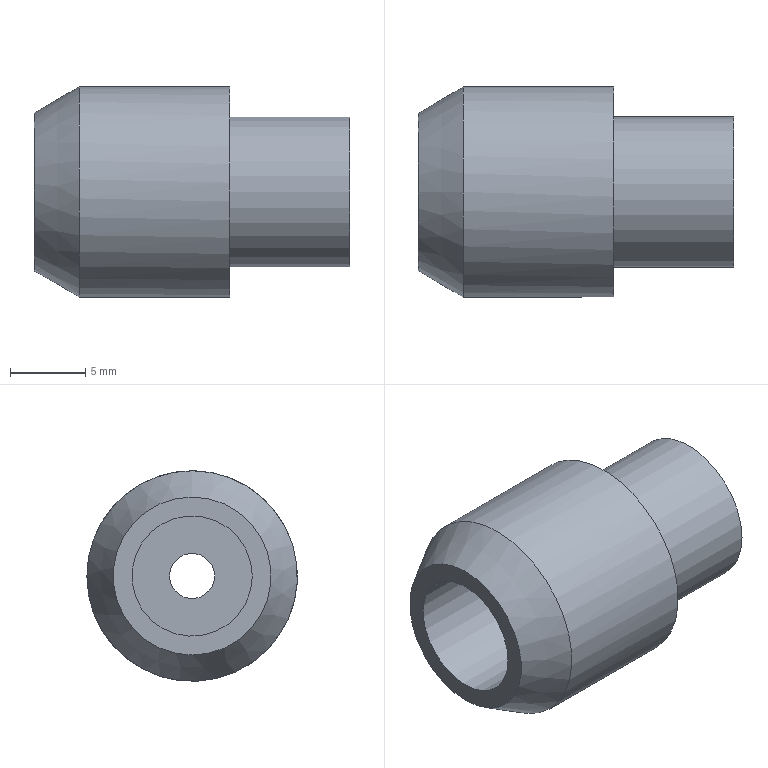Part | STEP file | 1-23.3 | 1 solid | 9 faces | box 21 x 14 x 14 mm | volume 1943 mm3 | cylinder 4 | plane 4 | cone 1 | commonest cylinder face diameters 3 x1 8 x1 10 x1 14 x1
STEP:
#1=CARTESIAN_POINT('',(0.,0.,0.));
#2=DIRECTION('',(0.,0.,1.));
#3=DIRECTION('',(1.,0.,0.));
#4=AXIS2_PLACEMENT_3D('',#1,#2,#3);
#5=CARTESIAN_POINT('',(0.,7.,0.));
#6=VERTEX_POINT('',#5);
#7=CARTESIAN_POINT('',(-10.,7.,0.));
#8=VERTEX_POINT('',#7);
#9=CARTESIAN_POINT('',(0.,7.,0.));
#10=DIRECTION('',(-1.,0.,0.));
#11=VECTOR('',#10,1.);
#12=LINE('',#9,#11);
#13=CARTESIAN_POINT('',(0.,0.,0.));
#14=DIRECTION('',(-1.,0.,0.));
#15=DIRECTION('',(0.,1.,0.));
#16=AXIS2_PLACEMENT_3D('',#13,#14,#15);
#17=CYLINDRICAL_SURFACE('',#16,7.);
#18=CARTESIAN_POINT('',(6.283,0.));
#19=DIRECTION('',(0.,1.));
#20=VECTOR('',#19,1.);
#21=LINE('',#18,#20);
#22=(GEOMETRIC_REPRESENTATION_CONTEXT(2)PARAMETRIC_REPRESENTATION_CONTEXT()REPRESENTATION_CONTEXT('',''));
#23=DEFINITIONAL_REPRESENTATION('',(#21),#22);
#24=PCURVE('',#17,#23);
#25=CARTESIAN_POINT('',(0.,0.));
#26=DIRECTION('',(0.,1.));
#27=VECTOR('',#26,1.);
#28=LINE('',#25,#27);
#29=(GEOMETRIC_REPRESENTATION_CONTEXT(2)PARAMETRIC_REPRESENTATION_CONTEXT()REPRESENTATION_CONTEXT('',''));
#30=DEFINITIONAL_REPRESENTATION('',(#28),#29);
#31=PCURVE('',#17,#30);
#32=SEAM_CURVE('',#12,(#24,#31),.PCURVE_S1.);
#33=EDGE_CURVE('',#6,#8,#32,.T.);
#34=ORIENTED_EDGE('',*,*,#33,.T.);
#35=CARTESIAN_POINT('',(-10.,0.,7.));
#36=VERTEX_POINT('',#35);
#37=CARTESIAN_POINT('',(-10.,0.,0.));
#38=DIRECTION('',(1.,0.,0.));
#39=DIRECTION('',(0.,1.,0.));
#40=AXIS2_PLACEMENT_3D('',#37,#38,#39);
#41=CIRCLE('',#40,7.);
#42=CARTESIAN_POINT('',(6.283,10.));
#43=DIRECTION('',(-1.,0.));
#44=VECTOR('',#43,1.);
#45=LINE('',#42,#44);
#46=(GEOMETRIC_REPRESENTATION_CONTEXT(2)PARAMETRIC_REPRESENTATION_CONTEXT()REPRESENTATION_CONTEXT('',''));
#47=DEFINITIONAL_REPRESENTATION('',(#45),#46);
#48=PCURVE('',#17,#47);
#49=CARTESIAN_POINT('',(-13.,0.,0.));
#50=DIRECTION('',(1.,0.,0.));
#51=DIRECTION('',(0.,0.,1.));
#52=AXIS2_PLACEMENT_3D('',#49,#50,#51);
#53=CONICAL_SURFACE('',#52,5.25,0.5281);
#54=CARTESIAN_POINT('',(4.712,3.));
#55=DIRECTION('',(1.,0.));
#56=VECTOR('',#55,1.);
#57=LINE('',#54,#56);
#58=(GEOMETRIC_REPRESENTATION_CONTEXT(2)PARAMETRIC_REPRESENTATION_CONTEXT()REPRESENTATION_CONTEXT('',''));
#59=DEFINITIONAL_REPRESENTATION('',(#57),#58);
#60=PCURVE('',#53,#59);
#61=SURFACE_CURVE('',#41,(#48,#60),.PCURVE_S1.);
#62=EDGE_CURVE('',#8,#36,#61,.T.);
#63=ORIENTED_EDGE('',*,*,#62,.T.);
#64=CARTESIAN_POINT('',(-10.,0.,0.));
#65=DIRECTION('',(1.,0.,0.));
#66=DIRECTION('',(0.,0.,1.));
#67=AXIS2_PLACEMENT_3D('',#64,#65,#66);
#68=CIRCLE('',#67,7.);
#69=CARTESIAN_POINT('',(4.712,10.));
#70=DIRECTION('',(-1.,0.));
#71=VECTOR('',#70,1.);
#72=LINE('',#69,#71);
#73=(GEOMETRIC_REPRESENTATION_CONTEXT(2)PARAMETRIC_REPRESENTATION_CONTEXT()REPRESENTATION_CONTEXT('',''));
#74=DEFINITIONAL_REPRESENTATION('',(#72),#73);
#75=PCURVE('',#17,#74);
#76=CARTESIAN_POINT('',(0.,3.));
#77=DIRECTION('',(1.,0.));
#78=VECTOR('',#77,1.);
#79=LINE('',#76,#78);
#80=(GEOMETRIC_REPRESENTATION_CONTEXT(2)PARAMETRIC_REPRESENTATION_CONTEXT()REPRESENTATION_CONTEXT('',''));
#81=DEFINITIONAL_REPRESENTATION('',(#79),#80);
#82=PCURVE('',#53,#81);
#83=SURFACE_CURVE('',#68,(#75,#82),.PCURVE_S1.);
#84=EDGE_CURVE('',#36,#8,#83,.T.);
#85=ORIENTED_EDGE('',*,*,#84,.T.);
#86=ORIENTED_EDGE('',*,*,#33,.F.);
#87=CARTESIAN_POINT('',(0.,0.,0.));
#88=DIRECTION('',(1.,0.,0.));
#89=DIRECTION('',(0.,1.,0.));
#90=AXIS2_PLACEMENT_3D('',#87,#88,#89);
#91=CIRCLE('',#90,7.);
#92=CARTESIAN_POINT('',(6.283,0.));
#93=DIRECTION('',(-1.,0.));
#94=VECTOR('',#93,1.);
#95=LINE('',#92,#94);
#96=(GEOMETRIC_REPRESENTATION_CONTEXT(2)PARAMETRIC_REPRESENTATION_CONTEXT()REPRESENTATION_CONTEXT('',''));
#97=DEFINITIONAL_REPRESENTATION('',(#95),#96);
#98=PCURVE('',#17,#97);
#99=CARTESIAN_POINT('',(0.,-1.876,0.));
#100=DIRECTION('',(1.,0.,0.));
#101=DIRECTION('',(0.,0.,-1.));
#102=AXIS2_PLACEMENT_3D('',#99,#100,#101);
#103=PLANE('',#102);
#104=CARTESIAN_POINT('',(0.,1.876));
#105=DIRECTION('',(0.,1.));
#106=AXIS2_PLACEMENT_2D('',#104,#105);
#107=CIRCLE('',#106,7.);
#108=(GEOMETRIC_REPRESENTATION_CONTEXT(2)PARAMETRIC_REPRESENTATION_CONTEXT()REPRESENTATION_CONTEXT('',''));
#109=DEFINITIONAL_REPRESENTATION('',(#107),#108);
#110=PCURVE('',#103,#109);
#111=SURFACE_CURVE('',#91,(#98,#110),.PCURVE_S1.);
#112=EDGE_CURVE('',#6,#6,#111,.T.);
#113=ORIENTED_EDGE('',*,*,#112,.F.);
#114=EDGE_LOOP('',(#34,#63,#85,#86,#113));
#115=FACE_BOUND('',#114,.T.);
#116=ADVANCED_FACE('',(#115),#17,.T.);
#117=ORIENTED_EDGE('',*,*,#112,.T.);
#118=EDGE_LOOP('',(#117));
#119=FACE_BOUND('',#118,.T.);
#120=CARTESIAN_POINT('',(0.,5.,0.));
#121=VERTEX_POINT('',#120);
#122=CARTESIAN_POINT('',(0.,0.,0.));
#123=DIRECTION('',(1.,0.,0.));
#124=DIRECTION('',(0.,1.,0.));
#125=AXIS2_PLACEMENT_3D('',#122,#123,#124);
#126=CIRCLE('',#125,5.);
#127=CARTESIAN_POINT('',(0.,1.876));
#128=DIRECTION('',(0.,1.));
#129=AXIS2_PLACEMENT_2D('',#127,#128);
#130=CIRCLE('',#129,5.);
#131=(GEOMETRIC_REPRESENTATION_CONTEXT(2)PARAMETRIC_REPRESENTATION_CONTEXT()REPRESENTATION_CONTEXT('',''));
#132=DEFINITIONAL_REPRESENTATION('',(#130),#131);
#133=PCURVE('',#103,#132);
#134=CARTESIAN_POINT('',(0.,0.,0.));
#135=DIRECTION('',(1.,0.,0.));
#136=DIRECTION('',(0.,1.,0.));
#137=AXIS2_PLACEMENT_3D('',#134,#135,#136);
#138=CYLINDRICAL_SURFACE('',#137,5.);
#139=CARTESIAN_POINT('',(0.,0.));
#140=DIRECTION('',(1.,0.));
#141=VECTOR('',#140,1.);
#142=LINE('',#139,#141);
#143=(GEOMETRIC_REPRESENTATION_CONTEXT(2)PARAMETRIC_REPRESENTATION_CONTEXT()REPRESENTATION_CONTEXT('',''));
#144=DEFINITIONAL_REPRESENTATION('',(#142),#143);
#145=PCURVE('',#138,#144);
#146=SURFACE_CURVE('',#126,(#133,#145),.PCURVE_S1.);
#147=EDGE_CURVE('',#121,#121,#146,.T.);
#148=ORIENTED_EDGE('',*,*,#147,.F.);
#149=EDGE_LOOP('',(#148));
#150=FACE_BOUND('',#149,.T.);
#151=ADVANCED_FACE('',(#119,#150),#103,.T.);
#152=ORIENTED_EDGE('',*,*,#147,.T.);
#153=CARTESIAN_POINT('',(8.,5.,0.));
#154=VERTEX_POINT('',#153);
#155=CARTESIAN_POINT('',(0.,5.,0.));
#156=DIRECTION('',(1.,0.,0.));
#157=VECTOR('',#156,1.);
#158=LINE('',#155,#157);
#159=CARTESIAN_POINT('',(6.283,0.));
#160=DIRECTION('',(0.,1.));
#161=VECTOR('',#160,1.);
#162=LINE('',#159,#161);
#163=(GEOMETRIC_REPRESENTATION_CONTEXT(2)PARAMETRIC_REPRESENTATION_CONTEXT()REPRESENTATION_CONTEXT('',''));
#164=DEFINITIONAL_REPRESENTATION('',(#162),#163);
#165=PCURVE('',#138,#164);
#166=CARTESIAN_POINT('',(0.,0.));
#167=DIRECTION('',(0.,1.));
#168=VECTOR('',#167,1.);
#169=LINE('',#166,#168);
#170=(GEOMETRIC_REPRESENTATION_CONTEXT(2)PARAMETRIC_REPRESENTATION_CONTEXT()REPRESENTATION_CONTEXT('',''));
#171=DEFINITIONAL_REPRESENTATION('',(#169),#170);
#172=PCURVE('',#138,#171);
#173=SEAM_CURVE('',#158,(#165,#172),.PCURVE_S1.);
#174=EDGE_CURVE('',#121,#154,#173,.T.);
#175=ORIENTED_EDGE('',*,*,#174,.T.);
#176=CARTESIAN_POINT('',(8.,0.,0.));
#177=DIRECTION('',(1.,0.,0.));
#178=DIRECTION('',(0.,1.,0.));
#179=AXIS2_PLACEMENT_3D('',#176,#177,#178);
#180=CIRCLE('',#179,5.);
#181=CARTESIAN_POINT('',(0.,8.));
#182=DIRECTION('',(1.,0.));
#183=VECTOR('',#182,1.);
#184=LINE('',#181,#183);
#185=(GEOMETRIC_REPRESENTATION_CONTEXT(2)PARAMETRIC_REPRESENTATION_CONTEXT()REPRESENTATION_CONTEXT('',''));
#186=DEFINITIONAL_REPRESENTATION('',(#184),#185);
#187=PCURVE('',#138,#186);
#188=CARTESIAN_POINT('',(8.,-1.34,0.));
#189=DIRECTION('',(1.,0.,0.));
#190=DIRECTION('',(0.,0.,-1.));
#191=AXIS2_PLACEMENT_3D('',#188,#189,#190);
#192=PLANE('',#191);
#193=CARTESIAN_POINT('',(0.,1.34));
#194=DIRECTION('',(0.,1.));
#195=AXIS2_PLACEMENT_2D('',#193,#194);
#196=CIRCLE('',#195,5.);
#197=(GEOMETRIC_REPRESENTATION_CONTEXT(2)PARAMETRIC_REPRESENTATION_CONTEXT()REPRESENTATION_CONTEXT('',''));
#198=DEFINITIONAL_REPRESENTATION('',(#196),#197);
#199=PCURVE('',#192,#198);
#200=SURFACE_CURVE('',#180,(#187,#199),.PCURVE_S1.);
#201=EDGE_CURVE('',#154,#154,#200,.T.);
#202=ORIENTED_EDGE('',*,*,#201,.F.);
#203=ORIENTED_EDGE('',*,*,#174,.F.);
#204=EDGE_LOOP('',(#152,#175,#202,#203));
#205=FACE_BOUND('',#204,.T.);
#206=ADVANCED_FACE('',(#205),#138,.T.);
#207=ORIENTED_EDGE('',*,*,#62,.F.);
#208=ORIENTED_EDGE('',*,*,#84,.F.);
#209=CARTESIAN_POINT('',(-13.,0.,5.25));
#210=VERTEX_POINT('',#209);
#211=CARTESIAN_POINT('',(-10.,0.,7.));
#212=DIRECTION('',(-0.8638,0.,-0.5039));
#213=VECTOR('',#212,1.);
#214=LINE('',#211,#213);
#215=CARTESIAN_POINT('',(0.,3.));
#216=DIRECTION('',(0.,-1.));
#217=VECTOR('',#216,1.);
#218=LINE('',#215,#217);
#219=(GEOMETRIC_REPRESENTATION_CONTEXT(2)PARAMETRIC_REPRESENTATION_CONTEXT()REPRESENTATION_CONTEXT('',''));
#220=DEFINITIONAL_REPRESENTATION('',(#218),#219);
#221=PCURVE('',#53,#220);
#222=CARTESIAN_POINT('',(6.283,3.));
#223=DIRECTION('',(0.,-1.));
#224=VECTOR('',#223,1.);
#225=LINE('',#222,#224);
#226=(GEOMETRIC_REPRESENTATION_CONTEXT(2)PARAMETRIC_REPRESENTATION_CONTEXT()REPRESENTATION_CONTEXT('',''));
#227=DEFINITIONAL_REPRESENTATION('',(#225),#226);
#228=PCURVE('',#53,#227);
#229=SEAM_CURVE('',#214,(#221,#228),.PCURVE_S1.);
#230=EDGE_CURVE('',#36,#210,#229,.T.);
#231=ORIENTED_EDGE('',*,*,#230,.T.);
#232=CARTESIAN_POINT('',(-13.,0.,0.));
#233=DIRECTION('',(-1.,0.,0.));
#234=DIRECTION('',(0.,0.,1.));
#235=AXIS2_PLACEMENT_3D('',#232,#233,#234);
#236=CIRCLE('',#235,5.25);
#237=CARTESIAN_POINT('',(6.283,0.));
#238=DIRECTION('',(-1.,0.));
#239=VECTOR('',#238,1.);
#240=LINE('',#237,#239);
#241=(GEOMETRIC_REPRESENTATION_CONTEXT(2)PARAMETRIC_REPRESENTATION_CONTEXT()REPRESENTATION_CONTEXT('',''));
#242=DEFINITIONAL_REPRESENTATION('',(#240),#241);
#243=PCURVE('',#53,#242);
#244=CARTESIAN_POINT('',(-13.,0.,0.));
#245=DIRECTION('',(1.,0.,0.));
#246=DIRECTION('',(0.,0.,1.));
#247=AXIS2_PLACEMENT_3D('',#244,#245,#246);
#248=PLANE('',#247);
#249=CARTESIAN_POINT('',(5.25,0.));
#250=CARTESIAN_POINT('',(5.25,-9.093));
#251=CARTESIAN_POINT('',(-2.625,-4.547));
#252=CARTESIAN_POINT('',(-10.5,0.));
#253=CARTESIAN_POINT('',(-2.625,4.547));
#254=CARTESIAN_POINT('',(5.25,9.093));
#255=CARTESIAN_POINT('',(5.25,0.));
#256=(BOUNDED_CURVE()B_SPLINE_CURVE(2,(#249,#250,#251,#252,#253,#254,#255),.UNSPECIFIED.,.T.,.F.)B_SPLINE_CURVE_WITH_KNOTS((1,2,2,2,2,1),(-2.094,0.,2.094,4.189,6.283,8.378),.UNSPECIFIED.)CURVE()GEOMETRIC_REPRESENTATION_ITEM()RATIONAL_B_SPLINE_CURVE((1.,0.5,1.,0.5,1.,0.5,1.))REPRESENTATION_ITEM(''));
#257=(GEOMETRIC_REPRESENTATION_CONTEXT(2)PARAMETRIC_REPRESENTATION_CONTEXT()REPRESENTATION_CONTEXT('',''));
#258=DEFINITIONAL_REPRESENTATION('',(#256),#257);
#259=PCURVE('',#248,#258);
#260=SURFACE_CURVE('',#236,(#243,#259),.PCURVE_S1.);
#261=EDGE_CURVE('',#210,#210,#260,.T.);
#262=ORIENTED_EDGE('',*,*,#261,.F.);
#263=ORIENTED_EDGE('',*,*,#230,.F.);
#264=EDGE_LOOP('',(#207,#208,#231,#262,#263));
#265=FACE_BOUND('',#264,.T.);
#266=ADVANCED_FACE('',(#265),#53,.T.);
#267=ORIENTED_EDGE('',*,*,#261,.F.);
#268=EDGE_LOOP('',(#267));
#269=FACE_BOUND('',#268,.F.);
#270=CARTESIAN_POINT('',(-13.,-4.,0.));
#271=VERTEX_POINT('',#270);
#272=CARTESIAN_POINT('',(-13.,0.,0.));
#273=DIRECTION('',(-1.,0.,0.));
#274=DIRECTION('',(0.,-1.,0.));
#275=AXIS2_PLACEMENT_3D('',#272,#273,#274);
#276=CIRCLE('',#275,4.);
#277=CARTESIAN_POINT('',(0.,4.));
#278=CARTESIAN_POINT('',(6.928,4.));
#279=CARTESIAN_POINT('',(3.464,-2.));
#280=CARTESIAN_POINT('',(0.,-8.));
#281=CARTESIAN_POINT('',(-3.464,-2.));
#282=CARTESIAN_POINT('',(-6.928,4.));
#283=CARTESIAN_POINT('',(0.,4.));
#284=(BOUNDED_CURVE()B_SPLINE_CURVE(2,(#277,#278,#279,#280,#281,#282,#283),.UNSPECIFIED.,.T.,.F.)B_SPLINE_CURVE_WITH_KNOTS((1,2,2,2,2,1),(-2.094,0.,2.094,4.189,6.283,8.378),.UNSPECIFIED.)CURVE()GEOMETRIC_REPRESENTATION_ITEM()RATIONAL_B_SPLINE_CURVE((1.,0.5,1.,0.5,1.,0.5,1.))REPRESENTATION_ITEM(''));
#285=(GEOMETRIC_REPRESENTATION_CONTEXT(2)PARAMETRIC_REPRESENTATION_CONTEXT()REPRESENTATION_CONTEXT('',''));
#286=DEFINITIONAL_REPRESENTATION('',(#284),#285);
#287=PCURVE('',#248,#286);
#288=CARTESIAN_POINT('',(-13.,0.,0.));
#289=DIRECTION('',(1.,0.,0.));
#290=DIRECTION('',(0.,-1.,0.));
#291=AXIS2_PLACEMENT_3D('',#288,#289,#290);
#292=CYLINDRICAL_SURFACE('',#291,4.);
#293=CARTESIAN_POINT('',(6.283,0.));
#294=DIRECTION('',(-1.,0.));
#295=VECTOR('',#294,1.);
#296=LINE('',#293,#295);
#297=(GEOMETRIC_REPRESENTATION_CONTEXT(2)PARAMETRIC_REPRESENTATION_CONTEXT()REPRESENTATION_CONTEXT('',''));
#298=DEFINITIONAL_REPRESENTATION('',(#296),#297);
#299=PCURVE('',#292,#298);
#300=SURFACE_CURVE('',#276,(#287,#299),.PCURVE_S1.);
#301=EDGE_CURVE('',#271,#271,#300,.T.);
#302=ORIENTED_EDGE('',*,*,#301,.T.);
#303=EDGE_LOOP('',(#302));
#304=FACE_BOUND('',#303,.F.);
#305=ADVANCED_FACE('',(#269,#304),#248,.F.);
#306=CARTESIAN_POINT('',(-3.,-4.,0.));
#307=VERTEX_POINT('',#306);
#308=CARTESIAN_POINT('',(-13.,-4.,0.));
#309=DIRECTION('',(1.,0.,0.));
#310=VECTOR('',#309,1.);
#311=LINE('',#308,#310);
#312=CARTESIAN_POINT('',(6.283,0.));
#313=DIRECTION('',(0.,1.));
#314=VECTOR('',#313,1.);
#315=LINE('',#312,#314);
#316=(GEOMETRIC_REPRESENTATION_CONTEXT(2)PARAMETRIC_REPRESENTATION_CONTEXT()REPRESENTATION_CONTEXT('',''));
#317=DEFINITIONAL_REPRESENTATION('',(#315),#316);
#318=PCURVE('',#292,#317);
#319=CARTESIAN_POINT('',(0.,0.));
#320=DIRECTION('',(0.,1.));
#321=VECTOR('',#320,1.);
#322=LINE('',#319,#321);
#323=(GEOMETRIC_REPRESENTATION_CONTEXT(2)PARAMETRIC_REPRESENTATION_CONTEXT()REPRESENTATION_CONTEXT('',''));
#324=DEFINITIONAL_REPRESENTATION('',(#322),#323);
#325=PCURVE('',#292,#324);
#326=SEAM_CURVE('',#311,(#318,#325),.PCURVE_S1.);
#327=EDGE_CURVE('',#271,#307,#326,.T.);
#328=ORIENTED_EDGE('',*,*,#327,.T.);
#329=CARTESIAN_POINT('',(-3.,0.,0.));
#330=DIRECTION('',(-1.,0.,0.));
#331=DIRECTION('',(0.,-1.,0.));
#332=AXIS2_PLACEMENT_3D('',#329,#330,#331);
#333=CIRCLE('',#332,4.);
#334=CARTESIAN_POINT('',(6.283,10.));
#335=DIRECTION('',(-1.,0.));
#336=VECTOR('',#335,1.);
#337=LINE('',#334,#336);
#338=(GEOMETRIC_REPRESENTATION_CONTEXT(2)PARAMETRIC_REPRESENTATION_CONTEXT()REPRESENTATION_CONTEXT('',''));
#339=DEFINITIONAL_REPRESENTATION('',(#337),#338);
#340=PCURVE('',#292,#339);
#341=CARTESIAN_POINT('',(-3.,1.072,0.));
#342=DIRECTION('',(-1.,0.,0.));
#343=DIRECTION('',(0.,-1.,0.));
#344=AXIS2_PLACEMENT_3D('',#341,#342,#343);
#345=PLANE('',#344);
#346=CARTESIAN_POINT('',(1.072,0.));
#347=DIRECTION('',(1.,0.));
#348=AXIS2_PLACEMENT_2D('',#346,#347);
#349=CIRCLE('',#348,4.);
#350=(GEOMETRIC_REPRESENTATION_CONTEXT(2)PARAMETRIC_REPRESENTATION_CONTEXT()REPRESENTATION_CONTEXT('',''));
#351=DEFINITIONAL_REPRESENTATION('',(#349),#350);
#352=PCURVE('',#345,#351);
#353=SURFACE_CURVE('',#333,(#340,#352),.PCURVE_S1.);
#354=EDGE_CURVE('',#307,#307,#353,.T.);
#355=ORIENTED_EDGE('',*,*,#354,.T.);
#356=ORIENTED_EDGE('',*,*,#327,.F.);
#357=ORIENTED_EDGE('',*,*,#301,.F.);
#358=EDGE_LOOP('',(#328,#355,#356,#357));
#359=FACE_BOUND('',#358,.F.);
#360=ADVANCED_FACE('',(#359),#292,.F.);
#361=ORIENTED_EDGE('',*,*,#201,.T.);
#362=EDGE_LOOP('',(#361));
#363=FACE_BOUND('',#362,.T.);
#364=CARTESIAN_POINT('',(8.,1.5,0.));
#365=VERTEX_POINT('',#364);
#366=CARTESIAN_POINT('',(8.,0.,0.));
#367=DIRECTION('',(1.,0.,0.));
#368=DIRECTION('',(0.,1.,0.));
#369=AXIS2_PLACEMENT_3D('',#366,#367,#368);
#370=CIRCLE('',#369,1.5);
#371=CARTESIAN_POINT('',(0.,1.34));
#372=DIRECTION('',(0.,1.));
#373=AXIS2_PLACEMENT_2D('',#371,#372);
#374=CIRCLE('',#373,1.5);
#375=(GEOMETRIC_REPRESENTATION_CONTEXT(2)PARAMETRIC_REPRESENTATION_CONTEXT()REPRESENTATION_CONTEXT('',''));
#376=DEFINITIONAL_REPRESENTATION('',(#374),#375);
#377=PCURVE('',#192,#376);
#378=CARTESIAN_POINT('',(8.,0.,0.));
#379=DIRECTION('',(-1.,0.,0.));
#380=DIRECTION('',(0.,1.,0.));
#381=AXIS2_PLACEMENT_3D('',#378,#379,#380);
#382=CYLINDRICAL_SURFACE('',#381,1.5);
#383=CARTESIAN_POINT('',(6.283,0.));
#384=DIRECTION('',(-1.,0.));
#385=VECTOR('',#384,1.);
#386=LINE('',#383,#385);
#387=(GEOMETRIC_REPRESENTATION_CONTEXT(2)PARAMETRIC_REPRESENTATION_CONTEXT()REPRESENTATION_CONTEXT('',''));
#388=DEFINITIONAL_REPRESENTATION('',(#386),#387);
#389=PCURVE('',#382,#388);
#390=SURFACE_CURVE('',#370,(#377,#389),.PCURVE_S1.);
#391=EDGE_CURVE('',#365,#365,#390,.T.);
#392=ORIENTED_EDGE('',*,*,#391,.F.);
#393=EDGE_LOOP('',(#392));
#394=FACE_BOUND('',#393,.T.);
#395=ADVANCED_FACE('',(#363,#394),#192,.T.);
#396=ORIENTED_EDGE('',*,*,#354,.T.);
#397=EDGE_LOOP('',(#396));
#398=FACE_BOUND('',#397,.T.);
#399=CARTESIAN_POINT('',(-3.,1.5,0.));
#400=VERTEX_POINT('',#399);
#401=CARTESIAN_POINT('',(-3.,0.,0.));
#402=DIRECTION('',(-1.,0.,0.));
#403=DIRECTION('',(0.,1.,0.));
#404=AXIS2_PLACEMENT_3D('',#401,#402,#403);
#405=CIRCLE('',#404,1.5);
#406=CARTESIAN_POINT('',(1.072,0.));
#407=DIRECTION('',(-1.,0.));
#408=AXIS2_PLACEMENT_2D('',#406,#407);
#409=CIRCLE('',#408,1.5);
#410=(GEOMETRIC_REPRESENTATION_CONTEXT(2)PARAMETRIC_REPRESENTATION_CONTEXT()REPRESENTATION_CONTEXT('',''));
#411=DEFINITIONAL_REPRESENTATION('',(#409),#410);
#412=PCURVE('',#345,#411);
#413=CARTESIAN_POINT('',(0.,11.));
#414=DIRECTION('',(1.,0.));
#415=VECTOR('',#414,1.);
#416=LINE('',#413,#415);
#417=(GEOMETRIC_REPRESENTATION_CONTEXT(2)PARAMETRIC_REPRESENTATION_CONTEXT()REPRESENTATION_CONTEXT('',''));
#418=DEFINITIONAL_REPRESENTATION('',(#416),#417);
#419=PCURVE('',#382,#418);
#420=SURFACE_CURVE('',#405,(#412,#419),.PCURVE_S1.);
#421=EDGE_CURVE('',#400,#400,#420,.T.);
#422=ORIENTED_EDGE('',*,*,#421,.F.);
#423=EDGE_LOOP('',(#422));
#424=FACE_BOUND('',#423,.T.);
#425=ADVANCED_FACE('',(#398,#424),#345,.T.);
#426=CARTESIAN_POINT('',(8.,1.5,0.));
#427=DIRECTION('',(-1.,0.,0.));
#428=VECTOR('',#427,1.);
#429=LINE('',#426,#428);
#430=CARTESIAN_POINT('',(6.283,0.));
#431=DIRECTION('',(0.,1.));
#432=VECTOR('',#431,1.);
#433=LINE('',#430,#432);
#434=(GEOMETRIC_REPRESENTATION_CONTEXT(2)PARAMETRIC_REPRESENTATION_CONTEXT()REPRESENTATION_CONTEXT('',''));
#435=DEFINITIONAL_REPRESENTATION('',(#433),#434);
#436=PCURVE('',#382,#435);
#437=CARTESIAN_POINT('',(0.,0.));
#438=DIRECTION('',(0.,1.));
#439=VECTOR('',#438,1.);
#440=LINE('',#437,#439);
#441=(GEOMETRIC_REPRESENTATION_CONTEXT(2)PARAMETRIC_REPRESENTATION_CONTEXT()REPRESENTATION_CONTEXT('',''));
#442=DEFINITIONAL_REPRESENTATION('',(#440),#441);
#443=PCURVE('',#382,#442);
#444=SEAM_CURVE('',#429,(#436,#443),.PCURVE_S1.);
#445=EDGE_CURVE('',#365,#400,#444,.T.);
#446=ORIENTED_EDGE('',*,*,#445,.T.);
#447=ORIENTED_EDGE('',*,*,#421,.F.);
#448=ORIENTED_EDGE('',*,*,#445,.F.);
#449=ORIENTED_EDGE('',*,*,#391,.F.);
#450=EDGE_LOOP('',(#446,#447,#448,#449));
#451=FACE_BOUND('',#450,.F.);
#452=ADVANCED_FACE('',(#451),#382,.F.);
#453=CLOSED_SHELL('',(#116,#151,#206,#266,#305,#360,#395,#425,#452));
#454=MANIFOLD_SOLID_BREP('',#453);
#455=(LENGTH_UNIT()NAMED_UNIT(*)SI_UNIT(.MILLI.,.METRE.));
#456=UNCERTAINTY_MEASURE_WITH_UNIT(LENGTH_MEASURE(0.0000001),#455,'','');
#457=(NAMED_UNIT(*)PLANE_ANGLE_UNIT()SI_UNIT($,.RADIAN.));
#458=(NAMED_UNIT(*)SI_UNIT($,.STERADIAN.)SOLID_ANGLE_UNIT());
#459=(GEOMETRIC_REPRESENTATION_CONTEXT(3)GLOBAL_UNCERTAINTY_ASSIGNED_CONTEXT((#456))GLOBAL_UNIT_ASSIGNED_CONTEXT((#455,#457,#458))REPRESENTATION_CONTEXT('',''));
#460=ADVANCED_BREP_SHAPE_REPRESENTATION('',(#4,#454),#459);